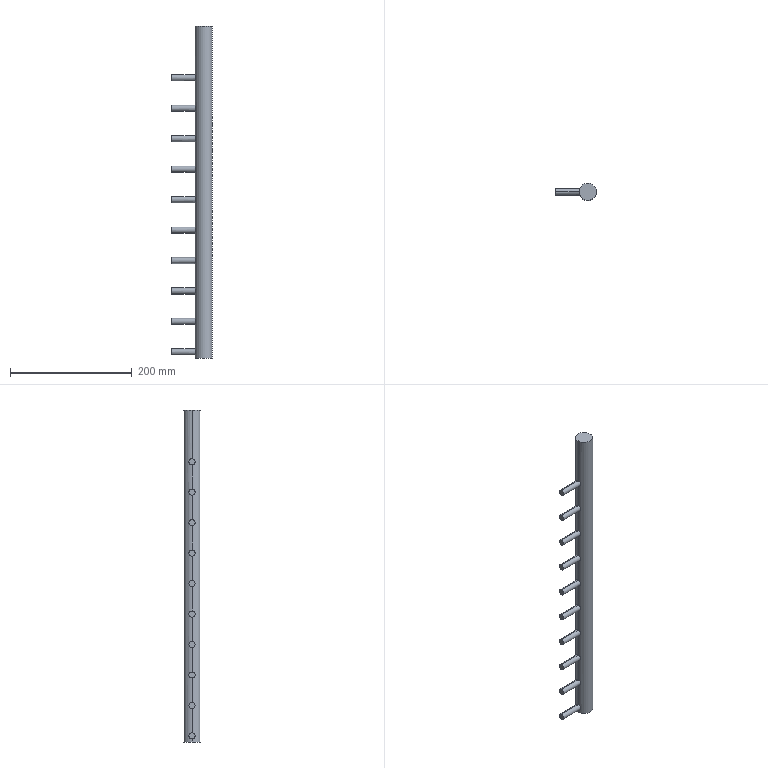Part | STEP file | part 161^COMPANY_A 408 evaporator | 1 solid | 34 faces | box 66.5 x 28 x 545 mm | volume 366001 mm3 | cylinder 22 | plane 12 | commonest cylinder face diameters 10 x20 28 x2